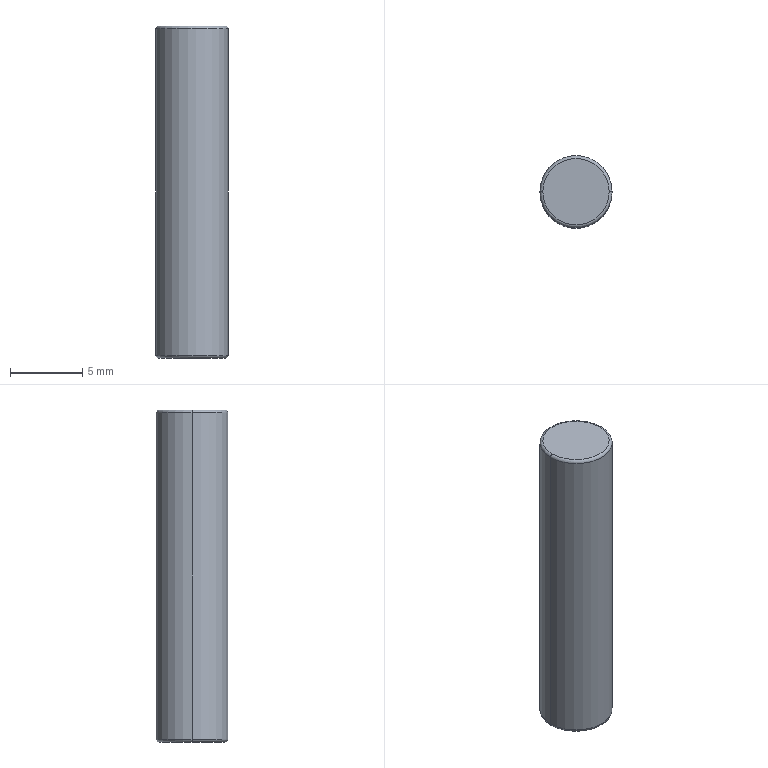Part | SolidWorks | features Extrusion 1, Fillet 1 | 1 solid | 8 faces | box 5 x 5 x 23 mm | volume 451.339 mm3 | torus 4 | cylinder 2 | plane 2 | commonest cylinder face diameters 5 x2
STEP:
#1=CARTESIAN_POINT('',(-2.5,0.,22.8));
#2=VERTEX_POINT('',#1);
#3=CARTESIAN_POINT('',(2.5,0.,22.8));
#4=VERTEX_POINT('',#3);
#5=CARTESIAN_POINT('',(0.,0.,22.8));
#6=DIRECTION('',(0.,0.,-1.));
#7=DIRECTION('',(1.,0.,0.));
#8=AXIS2_PLACEMENT_3D('',#5,#6,#7);
#9=CIRCLE('',#8,2.5);
#10=EDGE_CURVE('',#2,#4,#9,.T.);
#11=ORIENTED_EDGE('',*,*,#10,.F.);
#12=CARTESIAN_POINT('',(-2.3,0.,23.));
#13=VERTEX_POINT('',#12);
#14=CARTESIAN_POINT('',(-2.3,0.,22.8));
#15=DIRECTION('',(0.,1.,0.));
#16=DIRECTION('',(-1.,0.,0.));
#17=AXIS2_PLACEMENT_3D('',#14,#15,#16);
#18=CIRCLE('',#17,0.2);
#19=EDGE_CURVE('',#2,#13,#18,.T.);
#20=ORIENTED_EDGE('',*,*,#19,.T.);
#21=CARTESIAN_POINT('',(2.3,0.,23.));
#22=VERTEX_POINT('',#21);
#23=CARTESIAN_POINT('',(0.,0.,23.));
#24=DIRECTION('',(0.,0.,1.));
#25=DIRECTION('',(1.,0.,0.));
#26=AXIS2_PLACEMENT_3D('',#23,#24,#25);
#27=CIRCLE('',#26,2.3);
#28=EDGE_CURVE('',#22,#13,#27,.T.);
#29=ORIENTED_EDGE('',*,*,#28,.F.);
#30=CARTESIAN_POINT('',(2.3,0.,22.8));
#31=DIRECTION('',(0.,-1.,0.));
#32=DIRECTION('',(0.,0.,-1.));
#33=AXIS2_PLACEMENT_3D('',#30,#31,#32);
#34=CIRCLE('',#33,0.2);
#35=EDGE_CURVE('',#4,#22,#34,.T.);
#36=ORIENTED_EDGE('',*,*,#35,.F.);
#37=EDGE_LOOP('',(#11,#20,#29,#36));
#38=FACE_OUTER_BOUND('',#37,.T.);
#39=CARTESIAN_POINT('',(0.,0.,22.8));
#40=DIRECTION('',(0.,0.,1.));
#41=DIRECTION('',(1.,0.,0.));
#42=AXIS2_PLACEMENT_3D('',#39,#40,#41);
#43=TOROIDAL_SURFACE('',#42,2.3,0.2);
#44=ADVANCED_FACE('',(#38),#43,.T.);
#45=CARTESIAN_POINT('',(-2.3,0.,0.));
#46=VERTEX_POINT('',#45);
#47=CARTESIAN_POINT('',(2.3,0.,0.));
#48=VERTEX_POINT('',#47);
#49=CARTESIAN_POINT('',(0.,0.,0.));
#50=DIRECTION('',(0.,0.,-1.));
#51=DIRECTION('',(1.,0.,0.));
#52=AXIS2_PLACEMENT_3D('',#49,#50,#51);
#53=CIRCLE('',#52,2.3);
#54=EDGE_CURVE('',#46,#48,#53,.T.);
#55=ORIENTED_EDGE('',*,*,#54,.F.);
#56=CARTESIAN_POINT('',(-2.5,0.,0.2));
#57=VERTEX_POINT('',#56);
#58=CARTESIAN_POINT('',(-2.3,0.,0.2));
#59=DIRECTION('',(0.,1.,0.));
#60=DIRECTION('',(-1.,0.,0.));
#61=AXIS2_PLACEMENT_3D('',#58,#59,#60);
#62=CIRCLE('',#61,0.2);
#63=EDGE_CURVE('',#46,#57,#62,.T.);
#64=ORIENTED_EDGE('',*,*,#63,.T.);
#65=CARTESIAN_POINT('',(2.5,0.,0.2));
#66=VERTEX_POINT('',#65);
#67=CARTESIAN_POINT('',(0.,0.,0.2));
#68=DIRECTION('',(0.,0.,1.));
#69=DIRECTION('',(1.,0.,0.));
#70=AXIS2_PLACEMENT_3D('',#67,#68,#69);
#71=CIRCLE('',#70,2.5);
#72=EDGE_CURVE('',#66,#57,#71,.T.);
#73=ORIENTED_EDGE('',*,*,#72,.F.);
#74=CARTESIAN_POINT('',(2.3,0.,0.2));
#75=DIRECTION('',(0.,-1.,0.));
#76=DIRECTION('',(0.,0.,-1.));
#77=AXIS2_PLACEMENT_3D('',#74,#75,#76);
#78=CIRCLE('',#77,0.2);
#79=EDGE_CURVE('',#48,#66,#78,.T.);
#80=ORIENTED_EDGE('',*,*,#79,.F.);
#81=EDGE_LOOP('',(#55,#64,#73,#80));
#82=FACE_OUTER_BOUND('',#81,.T.);
#83=CARTESIAN_POINT('',(0.,0.,0.2));
#84=DIRECTION('',(0.,0.,1.));
#85=DIRECTION('',(1.,0.,0.));
#86=AXIS2_PLACEMENT_3D('',#83,#84,#85);
#87=TOROIDAL_SURFACE('',#86,2.3,0.2);
#88=ADVANCED_FACE('',(#82),#87,.T.);
#89=ORIENTED_EDGE('',*,*,#10,.T.);
#90=CARTESIAN_POINT('',(2.5,0.,23.));
#91=DIRECTION('',(0.,0.,-1.));
#92=VECTOR('',#91,1000.);
#93=LINE('',#90,#92);
#94=EDGE_CURVE('',#4,#66,#93,.T.);
#95=ORIENTED_EDGE('',*,*,#94,.T.);
#96=ORIENTED_EDGE('',*,*,#72,.T.);
#97=CARTESIAN_POINT('',(-2.5,0.,23.));
#98=DIRECTION('',(0.,0.,-1.));
#99=VECTOR('',#98,1000.);
#100=LINE('',#97,#99);
#101=EDGE_CURVE('',#2,#57,#100,.T.);
#102=ORIENTED_EDGE('',*,*,#101,.F.);
#103=EDGE_LOOP('',(#89,#95,#96,#102));
#104=FACE_OUTER_BOUND('',#103,.T.);
#105=CARTESIAN_POINT('',(0.,0.,23.));
#106=DIRECTION('',(0.,0.,-1.));
#107=DIRECTION('',(-1.,0.,0.));
#108=AXIS2_PLACEMENT_3D('',#105,#106,#107);
#109=CYLINDRICAL_SURFACE('',#108,2.5);
#110=ADVANCED_FACE('',(#104),#109,.T.);
#111=ORIENTED_EDGE('',*,*,#94,.F.);
#112=CARTESIAN_POINT('',(0.,0.,22.8));
#113=DIRECTION('',(0.,0.,-1.));
#114=DIRECTION('',(1.,0.,0.));
#115=AXIS2_PLACEMENT_3D('',#112,#113,#114);
#116=CIRCLE('',#115,2.5);
#117=EDGE_CURVE('',#4,#2,#116,.T.);
#118=ORIENTED_EDGE('',*,*,#117,.T.);
#119=ORIENTED_EDGE('',*,*,#101,.T.);
#120=CARTESIAN_POINT('',(0.,0.,0.2));
#121=DIRECTION('',(0.,0.,1.));
#122=DIRECTION('',(1.,0.,0.));
#123=AXIS2_PLACEMENT_3D('',#120,#121,#122);
#124=CIRCLE('',#123,2.5);
#125=EDGE_CURVE('',#57,#66,#124,.T.);
#126=ORIENTED_EDGE('',*,*,#125,.T.);
#127=EDGE_LOOP('',(#111,#118,#119,#126));
#128=FACE_OUTER_BOUND('',#127,.T.);
#129=CARTESIAN_POINT('',(0.,0.,23.));
#130=DIRECTION('',(0.,0.,-1.));
#131=DIRECTION('',(-1.,0.,0.));
#132=AXIS2_PLACEMENT_3D('',#129,#130,#131);
#133=CYLINDRICAL_SURFACE('',#132,2.5);
#134=ADVANCED_FACE('',(#128),#133,.T.);
#135=ORIENTED_EDGE('',*,*,#28,.T.);
#136=CARTESIAN_POINT('',(0.,0.,23.));
#137=DIRECTION('',(0.,0.,1.));
#138=DIRECTION('',(1.,0.,0.));
#139=AXIS2_PLACEMENT_3D('',#136,#137,#138);
#140=CIRCLE('',#139,2.3);
#141=EDGE_CURVE('',#13,#22,#140,.T.);
#142=ORIENTED_EDGE('',*,*,#141,.T.);
#143=EDGE_LOOP('',(#135,#142));
#144=FACE_OUTER_BOUND('',#143,.T.);
#145=CARTESIAN_POINT('',(0.,0.,23.));
#146=DIRECTION('',(0.,0.,1.));
#147=DIRECTION('',(1.,0.,0.));
#148=AXIS2_PLACEMENT_3D('',#145,#146,#147);
#149=PLANE('',#148);
#150=ADVANCED_FACE('',(#144),#149,.T.);
#151=CARTESIAN_POINT('',(0.,0.,0.));
#152=DIRECTION('',(0.,0.,-1.));
#153=DIRECTION('',(1.,0.,0.));
#154=AXIS2_PLACEMENT_3D('',#151,#152,#153);
#155=CIRCLE('',#154,2.3);
#156=EDGE_CURVE('',#48,#46,#155,.T.);
#157=ORIENTED_EDGE('',*,*,#156,.T.);
#158=ORIENTED_EDGE('',*,*,#54,.T.);
#159=EDGE_LOOP('',(#157,#158));
#160=FACE_OUTER_BOUND('',#159,.T.);
#161=CARTESIAN_POINT('',(0.,0.,0.));
#162=DIRECTION('',(0.,0.,1.));
#163=DIRECTION('',(1.,0.,0.));
#164=AXIS2_PLACEMENT_3D('',#161,#162,#163);
#165=PLANE('',#164);
#166=ADVANCED_FACE('',(#160),#165,.F.);
#167=ORIENTED_EDGE('',*,*,#63,.F.);
#168=ORIENTED_EDGE('',*,*,#156,.F.);
#169=ORIENTED_EDGE('',*,*,#79,.T.);
#170=ORIENTED_EDGE('',*,*,#125,.F.);
#171=EDGE_LOOP('',(#167,#168,#169,#170));
#172=FACE_OUTER_BOUND('',#171,.T.);
#173=CARTESIAN_POINT('',(0.,0.,0.2));
#174=DIRECTION('',(0.,0.,1.));
#175=DIRECTION('',(1.,0.,0.));
#176=AXIS2_PLACEMENT_3D('',#173,#174,#175);
#177=TOROIDAL_SURFACE('',#176,2.3,0.2);
#178=ADVANCED_FACE('',(#172),#177,.T.);
#179=ORIENTED_EDGE('',*,*,#19,.F.);
#180=ORIENTED_EDGE('',*,*,#117,.F.);
#181=ORIENTED_EDGE('',*,*,#35,.T.);
#182=ORIENTED_EDGE('',*,*,#141,.F.);
#183=EDGE_LOOP('',(#179,#180,#181,#182));
#184=FACE_OUTER_BOUND('',#183,.T.);
#185=CARTESIAN_POINT('',(0.,0.,22.8));
#186=DIRECTION('',(0.,0.,1.));
#187=DIRECTION('',(1.,0.,0.));
#188=AXIS2_PLACEMENT_3D('',#185,#186,#187);
#189=TOROIDAL_SURFACE('',#188,2.3,0.2);
#190=ADVANCED_FACE('',(#184),#189,.T.);
#191=CLOSED_SHELL('',(#44,#88,#110,#134,#150,#166,#178,#190));
#192=MANIFOLD_SOLID_BREP('',#191);
#193=CARTESIAN_POINT('',(0.,0.,0.));
#194=DIRECTION('',(0.,0.,1.));
#195=DIRECTION('',(1.,0.,0.));
#196=AXIS2_PLACEMENT_3D('',#193,#194,#195);
#197=(LENGTH_UNIT()NAMED_UNIT(*)SI_UNIT(.MILLI.,.METRE.));
#198=UNCERTAINTY_MEASURE_WITH_UNIT(LENGTH_MEASURE(0.00001),#197,'','');
#199=(NAMED_UNIT(*)PLANE_ANGLE_UNIT()SI_UNIT($,.RADIAN.));
#200=(NAMED_UNIT(*)SI_UNIT($,.STERADIAN.)SOLID_ANGLE_UNIT());
#201=(GEOMETRIC_REPRESENTATION_CONTEXT(3)GLOBAL_UNCERTAINTY_ASSIGNED_CONTEXT((#198))GLOBAL_UNIT_ASSIGNED_CONTEXT((#197,#199,#200))REPRESENTATION_CONTEXT('',''));
#202=ADVANCED_BREP_SHAPE_REPRESENTATION('',(#192,#196),#201);